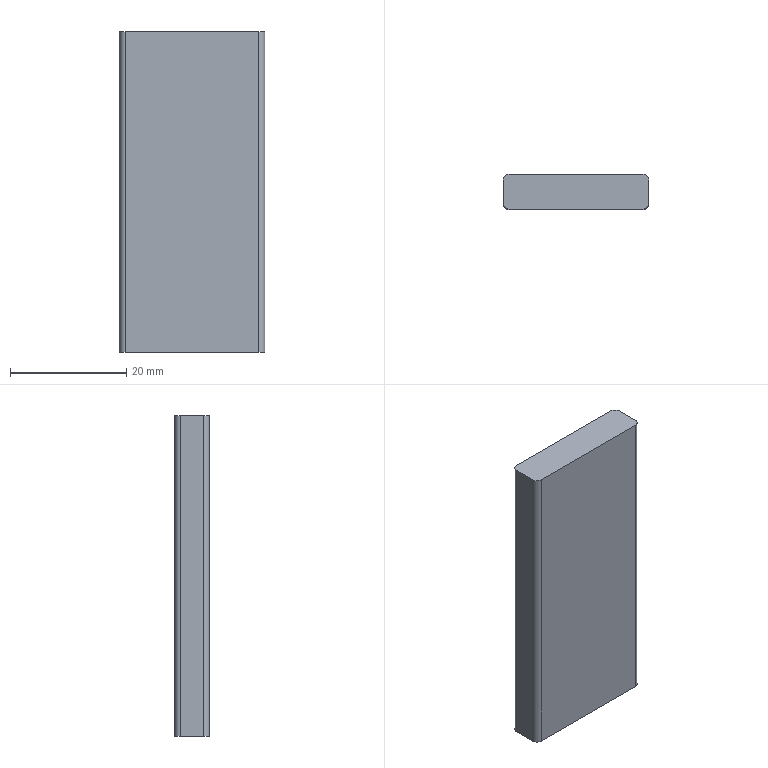Part | STEP file | 1 solid | 10 faces | box 24.97 x 5.97 x 55 mm | volume 8152 mm3 | plane 6 | cylinder 4 | commonest cylinder face diameters 2 x4
STEP:
#1=CARTESIAN_POINT('',(0.,0.,0.));
#2=DIRECTION('',(0.,0.,1.));
#3=DIRECTION('',(1.,0.,0.));
#4=AXIS2_PLACEMENT_3D('',#1,#2,#3);
#5=CARTESIAN_POINT('',(1790.232,496.365,31.619));
#6=VERTEX_POINT('',#5);
#7=CARTESIAN_POINT('',(1767.262,496.365,31.619));
#8=VERTEX_POINT('',#7);
#9=CARTESIAN_POINT('',(1791.247,496.365,31.619));
#10=DIRECTION('',(-1.,0.,0.));
#11=VECTOR('',#10,1.);
#12=LINE('',#9,#11);
#13=CARTESIAN_POINT('',(1801.247,562.98,31.619));
#14=DIRECTION('',(0.,0.,-1.));
#15=DIRECTION('',(-1.,0.,0.));
#16=AXIS2_PLACEMENT_3D('',#13,#14,#15);
#17=PLANE('',#16);
#18=CARTESIAN_POINT('',(10.,-66.615));
#19=DIRECTION('',(1.,0.));
#20=VECTOR('',#19,1.);
#21=LINE('',#18,#20);
#22=(GEOMETRIC_REPRESENTATION_CONTEXT(2)PARAMETRIC_REPRESENTATION_CONTEXT()REPRESENTATION_CONTEXT('',''));
#23=DEFINITIONAL_REPRESENTATION('',(#21),#22);
#24=PCURVE('',#17,#23);
#25=CARTESIAN_POINT('',(1791.247,496.365,426.119));
#26=DIRECTION('',(0.,-1.,0.));
#27=DIRECTION('',(0.,0.,1.));
#28=AXIS2_PLACEMENT_3D('',#25,#26,#27);
#29=PLANE('',#28);
#30=CARTESIAN_POINT('',(-394.5,0.));
#31=DIRECTION('',(0.,1.));
#32=VECTOR('',#31,1.);
#33=LINE('',#30,#32);
#34=(GEOMETRIC_REPRESENTATION_CONTEXT(2)PARAMETRIC_REPRESENTATION_CONTEXT()REPRESENTATION_CONTEXT('',''));
#35=DEFINITIONAL_REPRESENTATION('',(#33),#34);
#36=PCURVE('',#29,#35);
#37=SURFACE_CURVE('',#12,(#24,#36),.PCURVE_S1.);
#38=EDGE_CURVE('',#6,#8,#37,.T.);
#39=ORIENTED_EDGE('',*,*,#38,.T.);
#40=CARTESIAN_POINT('',(1766.262,495.365,31.619));
#41=VERTEX_POINT('',#40);
#42=CARTESIAN_POINT('',(1767.262,495.365,31.619));
#43=DIRECTION('',(0.,0.,1.));
#44=DIRECTION('',(-1.,0.,0.));
#45=AXIS2_PLACEMENT_3D('',#42,#43,#44);
#46=CIRCLE('',#45,1.);
#47=CARTESIAN_POINT('',(34.985,-67.615));
#48=CARTESIAN_POINT('',(34.985,-69.347));
#49=CARTESIAN_POINT('',(33.485,-68.481));
#50=CARTESIAN_POINT('',(31.985,-67.615));
#51=CARTESIAN_POINT('',(33.485,-66.749));
#52=CARTESIAN_POINT('',(34.985,-65.883));
#53=CARTESIAN_POINT('',(34.985,-67.615));
#54=(BOUNDED_CURVE()B_SPLINE_CURVE(2,(#47,#48,#49,#50,#51,#52,#53),.UNSPECIFIED.,.T.,.F.)B_SPLINE_CURVE_WITH_KNOTS((1,2,2,2,2,1),(-2.094,0.,2.094,4.189,6.283,8.378),.UNSPECIFIED.)CURVE()GEOMETRIC_REPRESENTATION_ITEM()RATIONAL_B_SPLINE_CURVE((1.,0.5,1.,0.5,1.,0.5,1.))REPRESENTATION_ITEM(''));
#55=(GEOMETRIC_REPRESENTATION_CONTEXT(2)PARAMETRIC_REPRESENTATION_CONTEXT()REPRESENTATION_CONTEXT('',''));
#56=DEFINITIONAL_REPRESENTATION('',(#54),#55);
#57=PCURVE('',#17,#56);
#58=CARTESIAN_POINT('',(1767.262,495.365,426.119));
#59=DIRECTION('',(0.,0.,-1.));
#60=DIRECTION('',(-1.,0.,0.));
#61=AXIS2_PLACEMENT_3D('',#58,#59,#60);
#62=CYLINDRICAL_SURFACE('',#61,1.);
#63=CARTESIAN_POINT('',(6.283,394.5));
#64=DIRECTION('',(-1.,0.));
#65=VECTOR('',#64,1.);
#66=LINE('',#63,#65);
#67=(GEOMETRIC_REPRESENTATION_CONTEXT(2)PARAMETRIC_REPRESENTATION_CONTEXT()REPRESENTATION_CONTEXT('',''));
#68=DEFINITIONAL_REPRESENTATION('',(#66),#67);
#69=PCURVE('',#62,#68);
#70=SURFACE_CURVE('',#46,(#57,#69),.PCURVE_S1.);
#71=EDGE_CURVE('',#8,#41,#70,.T.);
#72=ORIENTED_EDGE('',*,*,#71,.T.);
#73=CARTESIAN_POINT('',(1766.262,491.395,31.619));
#74=VERTEX_POINT('',#73);
#75=CARTESIAN_POINT('',(1766.262,496.38,31.619));
#76=DIRECTION('',(0.,-1.,0.));
#77=VECTOR('',#76,1.);
#78=LINE('',#75,#77);
#79=CARTESIAN_POINT('',(34.985,-66.6));
#80=DIRECTION('',(0.,-1.));
#81=VECTOR('',#80,1.);
#82=LINE('',#79,#81);
#83=(GEOMETRIC_REPRESENTATION_CONTEXT(2)PARAMETRIC_REPRESENTATION_CONTEXT()REPRESENTATION_CONTEXT('',''));
#84=DEFINITIONAL_REPRESENTATION('',(#82),#83);
#85=PCURVE('',#17,#84);
#86=CARTESIAN_POINT('',(1766.262,496.38,426.119));
#87=DIRECTION('',(1.,0.,0.));
#88=DIRECTION('',(0.,0.,-1.));
#89=AXIS2_PLACEMENT_3D('',#86,#87,#88);
#90=PLANE('',#89);
#91=CARTESIAN_POINT('',(394.5,0.));
#92=DIRECTION('',(0.,-1.));
#93=VECTOR('',#92,1.);
#94=LINE('',#91,#93);
#95=(GEOMETRIC_REPRESENTATION_CONTEXT(2)PARAMETRIC_REPRESENTATION_CONTEXT()REPRESENTATION_CONTEXT('',''));
#96=DEFINITIONAL_REPRESENTATION('',(#94),#95);
#97=PCURVE('',#90,#96);
#98=SURFACE_CURVE('',#78,(#85,#97),.PCURVE_S1.);
#99=EDGE_CURVE('',#41,#74,#98,.T.);
#100=ORIENTED_EDGE('',*,*,#99,.T.);
#101=CARTESIAN_POINT('',(1767.262,490.395,31.619));
#102=VERTEX_POINT('',#101);
#103=CARTESIAN_POINT('',(1767.262,491.395,31.619));
#104=DIRECTION('',(0.,0.,1.));
#105=DIRECTION('',(-1.,0.,0.));
#106=AXIS2_PLACEMENT_3D('',#103,#104,#105);
#107=CIRCLE('',#106,1.);
#108=CARTESIAN_POINT('',(34.985,-71.585));
#109=CARTESIAN_POINT('',(34.985,-73.317));
#110=CARTESIAN_POINT('',(33.485,-72.451));
#111=CARTESIAN_POINT('',(31.985,-71.585));
#112=CARTESIAN_POINT('',(33.485,-70.719));
#113=CARTESIAN_POINT('',(34.985,-69.853));
#114=CARTESIAN_POINT('',(34.985,-71.585));
#115=(BOUNDED_CURVE()B_SPLINE_CURVE(2,(#108,#109,#110,#111,#112,#113,#114),.UNSPECIFIED.,.T.,.F.)B_SPLINE_CURVE_WITH_KNOTS((1,2,2,2,2,1),(-2.094,0.,2.094,4.189,6.283,8.378),.UNSPECIFIED.)CURVE()GEOMETRIC_REPRESENTATION_ITEM()RATIONAL_B_SPLINE_CURVE((1.,0.5,1.,0.5,1.,0.5,1.))REPRESENTATION_ITEM(''));
#116=(GEOMETRIC_REPRESENTATION_CONTEXT(2)PARAMETRIC_REPRESENTATION_CONTEXT()REPRESENTATION_CONTEXT('',''));
#117=DEFINITIONAL_REPRESENTATION('',(#115),#116);
#118=PCURVE('',#17,#117);
#119=CARTESIAN_POINT('',(1767.262,491.395,426.119));
#120=DIRECTION('',(0.,0.,-1.));
#121=DIRECTION('',(-1.,0.,0.));
#122=AXIS2_PLACEMENT_3D('',#119,#120,#121);
#123=CYLINDRICAL_SURFACE('',#122,1.);
#124=CARTESIAN_POINT('',(6.283,394.5));
#125=DIRECTION('',(-1.,0.));
#126=VECTOR('',#125,1.);
#127=LINE('',#124,#126);
#128=(GEOMETRIC_REPRESENTATION_CONTEXT(2)PARAMETRIC_REPRESENTATION_CONTEXT()REPRESENTATION_CONTEXT('',''));
#129=DEFINITIONAL_REPRESENTATION('',(#127),#128);
#130=PCURVE('',#123,#129);
#131=SURFACE_CURVE('',#107,(#118,#130),.PCURVE_S1.);
#132=EDGE_CURVE('',#74,#102,#131,.T.);
#133=ORIENTED_EDGE('',*,*,#132,.T.);
#134=CARTESIAN_POINT('',(1790.232,490.395,31.619));
#135=VERTEX_POINT('',#134);
#136=CARTESIAN_POINT('',(1761.247,490.395,31.619));
#137=DIRECTION('',(1.,0.,0.));
#138=VECTOR('',#137,1.);
#139=LINE('',#136,#138);
#140=CARTESIAN_POINT('',(40.,-72.585));
#141=DIRECTION('',(-1.,0.));
#142=VECTOR('',#141,1.);
#143=LINE('',#140,#142);
#144=(GEOMETRIC_REPRESENTATION_CONTEXT(2)PARAMETRIC_REPRESENTATION_CONTEXT()REPRESENTATION_CONTEXT('',''));
#145=DEFINITIONAL_REPRESENTATION('',(#143),#144);
#146=PCURVE('',#17,#145);
#147=CARTESIAN_POINT('',(1761.247,490.395,426.119));
#148=DIRECTION('',(0.,1.,0.));
#149=DIRECTION('',(0.,0.,-1.));
#150=AXIS2_PLACEMENT_3D('',#147,#148,#149);
#151=PLANE('',#150);
#152=CARTESIAN_POINT('',(394.5,0.));
#153=DIRECTION('',(0.,-1.));
#154=VECTOR('',#153,1.);
#155=LINE('',#152,#154);
#156=(GEOMETRIC_REPRESENTATION_CONTEXT(2)PARAMETRIC_REPRESENTATION_CONTEXT()REPRESENTATION_CONTEXT('',''));
#157=DEFINITIONAL_REPRESENTATION('',(#155),#156);
#158=PCURVE('',#151,#157);
#159=SURFACE_CURVE('',#139,(#146,#158),.PCURVE_S1.);
#160=EDGE_CURVE('',#102,#135,#159,.T.);
#161=ORIENTED_EDGE('',*,*,#160,.T.);
#162=CARTESIAN_POINT('',(1791.232,491.395,31.619));
#163=VERTEX_POINT('',#162);
#164=CARTESIAN_POINT('',(1790.232,491.395,31.619));
#165=DIRECTION('',(0.,0.,1.));
#166=DIRECTION('',(-1.,0.,0.));
#167=AXIS2_PLACEMENT_3D('',#164,#165,#166);
#168=CIRCLE('',#167,1.);
#169=CARTESIAN_POINT('',(12.015,-71.585));
#170=CARTESIAN_POINT('',(12.015,-73.317));
#171=CARTESIAN_POINT('',(10.515,-72.451));
#172=CARTESIAN_POINT('',(9.015,-71.585));
#173=CARTESIAN_POINT('',(10.515,-70.719));
#174=CARTESIAN_POINT('',(12.015,-69.853));
#175=CARTESIAN_POINT('',(12.015,-71.585));
#176=(BOUNDED_CURVE()B_SPLINE_CURVE(2,(#169,#170,#171,#172,#173,#174,#175),.UNSPECIFIED.,.T.,.F.)B_SPLINE_CURVE_WITH_KNOTS((1,2,2,2,2,1),(-2.094,0.,2.094,4.189,6.283,8.378),.UNSPECIFIED.)CURVE()GEOMETRIC_REPRESENTATION_ITEM()RATIONAL_B_SPLINE_CURVE((1.,0.5,1.,0.5,1.,0.5,1.))REPRESENTATION_ITEM(''));
#177=(GEOMETRIC_REPRESENTATION_CONTEXT(2)PARAMETRIC_REPRESENTATION_CONTEXT()REPRESENTATION_CONTEXT('',''));
#178=DEFINITIONAL_REPRESENTATION('',(#176),#177);
#179=PCURVE('',#17,#178);
#180=CARTESIAN_POINT('',(1790.232,491.395,426.119));
#181=DIRECTION('',(0.,0.,-1.));
#182=DIRECTION('',(-1.,0.,0.));
#183=AXIS2_PLACEMENT_3D('',#180,#181,#182);
#184=CYLINDRICAL_SURFACE('',#183,1.);
#185=CARTESIAN_POINT('',(6.283,394.5));
#186=DIRECTION('',(-1.,0.));
#187=VECTOR('',#186,1.);
#188=LINE('',#185,#187);
#189=(GEOMETRIC_REPRESENTATION_CONTEXT(2)PARAMETRIC_REPRESENTATION_CONTEXT()REPRESENTATION_CONTEXT('',''));
#190=DEFINITIONAL_REPRESENTATION('',(#188),#189);
#191=PCURVE('',#184,#190);
#192=SURFACE_CURVE('',#168,(#179,#191),.PCURVE_S1.);
#193=EDGE_CURVE('',#135,#163,#192,.T.);
#194=ORIENTED_EDGE('',*,*,#193,.T.);
#195=CARTESIAN_POINT('',(1791.232,495.365,31.619));
#196=VERTEX_POINT('',#195);
#197=CARTESIAN_POINT('',(1791.232,490.38,31.619));
#198=DIRECTION('',(0.,1.,0.));
#199=VECTOR('',#198,1.);
#200=LINE('',#197,#199);
#201=CARTESIAN_POINT('',(10.015,-72.6));
#202=DIRECTION('',(0.,1.));
#203=VECTOR('',#202,1.);
#204=LINE('',#201,#203);
#205=(GEOMETRIC_REPRESENTATION_CONTEXT(2)PARAMETRIC_REPRESENTATION_CONTEXT()REPRESENTATION_CONTEXT('',''));
#206=DEFINITIONAL_REPRESENTATION('',(#204),#205);
#207=PCURVE('',#17,#206);
#208=CARTESIAN_POINT('',(1791.232,490.38,426.119));
#209=DIRECTION('',(-1.,0.,0.));
#210=DIRECTION('',(0.,0.,1.));
#211=AXIS2_PLACEMENT_3D('',#208,#209,#210);
#212=PLANE('',#211);
#213=CARTESIAN_POINT('',(-394.5,0.));
#214=DIRECTION('',(0.,1.));
#215=VECTOR('',#214,1.);
#216=LINE('',#213,#215);
#217=(GEOMETRIC_REPRESENTATION_CONTEXT(2)PARAMETRIC_REPRESENTATION_CONTEXT()REPRESENTATION_CONTEXT('',''));
#218=DEFINITIONAL_REPRESENTATION('',(#216),#217);
#219=PCURVE('',#212,#218);
#220=SURFACE_CURVE('',#200,(#207,#219),.PCURVE_S1.);
#221=EDGE_CURVE('',#163,#196,#220,.T.);
#222=ORIENTED_EDGE('',*,*,#221,.T.);
#223=CARTESIAN_POINT('',(1790.232,495.365,31.619));
#224=DIRECTION('',(0.,0.,1.));
#225=DIRECTION('',(-1.,0.,0.));
#226=AXIS2_PLACEMENT_3D('',#223,#224,#225);
#227=CIRCLE('',#226,1.);
#228=CARTESIAN_POINT('',(12.015,-67.615));
#229=CARTESIAN_POINT('',(12.015,-69.347));
#230=CARTESIAN_POINT('',(10.515,-68.481));
#231=CARTESIAN_POINT('',(9.015,-67.615));
#232=CARTESIAN_POINT('',(10.515,-66.749));
#233=CARTESIAN_POINT('',(12.015,-65.883));
#234=CARTESIAN_POINT('',(12.015,-67.615));
#235=(BOUNDED_CURVE()B_SPLINE_CURVE(2,(#228,#229,#230,#231,#232,#233,#234),.UNSPECIFIED.,.T.,.F.)B_SPLINE_CURVE_WITH_KNOTS((1,2,2,2,2,1),(-2.094,0.,2.094,4.189,6.283,8.378),.UNSPECIFIED.)CURVE()GEOMETRIC_REPRESENTATION_ITEM()RATIONAL_B_SPLINE_CURVE((1.,0.5,1.,0.5,1.,0.5,1.))REPRESENTATION_ITEM(''));
#236=(GEOMETRIC_REPRESENTATION_CONTEXT(2)PARAMETRIC_REPRESENTATION_CONTEXT()REPRESENTATION_CONTEXT('',''));
#237=DEFINITIONAL_REPRESENTATION('',(#235),#236);
#238=PCURVE('',#17,#237);
#239=CARTESIAN_POINT('',(1790.232,495.365,426.119));
#240=DIRECTION('',(0.,0.,-1.));
#241=DIRECTION('',(-1.,0.,0.));
#242=AXIS2_PLACEMENT_3D('',#239,#240,#241);
#243=CYLINDRICAL_SURFACE('',#242,1.);
#244=CARTESIAN_POINT('',(6.283,394.5));
#245=DIRECTION('',(-1.,0.));
#246=VECTOR('',#245,1.);
#247=LINE('',#244,#246);
#248=(GEOMETRIC_REPRESENTATION_CONTEXT(2)PARAMETRIC_REPRESENTATION_CONTEXT()REPRESENTATION_CONTEXT('',''));
#249=DEFINITIONAL_REPRESENTATION('',(#247),#248);
#250=PCURVE('',#243,#249);
#251=SURFACE_CURVE('',#227,(#238,#250),.PCURVE_S1.);
#252=EDGE_CURVE('',#196,#6,#251,.T.);
#253=ORIENTED_EDGE('',*,*,#252,.T.);
#254=EDGE_LOOP('',(#39,#72,#100,#133,#161,#194,#222,#253));
#255=FACE_BOUND('',#254,.T.);
#256=ADVANCED_FACE('',(#255),#17,.F.);
#257=CARTESIAN_POINT('',(1790.232,496.365,-23.381));
#258=VERTEX_POINT('',#257);
#259=CARTESIAN_POINT('',(1767.262,496.365,-23.381));
#260=VERTEX_POINT('',#259);
#261=CARTESIAN_POINT('',(1791.247,496.365,-23.381));
#262=DIRECTION('',(-1.,0.,0.));
#263=VECTOR('',#262,1.);
#264=LINE('',#261,#263);
#265=CARTESIAN_POINT('',(-449.5,0.));
#266=DIRECTION('',(0.,1.));
#267=VECTOR('',#266,1.);
#268=LINE('',#265,#267);
#269=(GEOMETRIC_REPRESENTATION_CONTEXT(2)PARAMETRIC_REPRESENTATION_CONTEXT()REPRESENTATION_CONTEXT('',''));
#270=DEFINITIONAL_REPRESENTATION('',(#268),#269);
#271=PCURVE('',#29,#270);
#272=CARTESIAN_POINT('',(18956.132,-3517.479,-23.381));
#273=DIRECTION('',(0.,0.,1.));
#274=DIRECTION('',(1.,0.,0.));
#275=AXIS2_PLACEMENT_3D('',#272,#273,#274);
#276=PLANE('',#275);
#277=CARTESIAN_POINT('',(-17164.884,4013.844));
#278=DIRECTION('',(-1.,0.));
#279=VECTOR('',#278,1.);
#280=LINE('',#277,#279);
#281=(GEOMETRIC_REPRESENTATION_CONTEXT(2)PARAMETRIC_REPRESENTATION_CONTEXT()REPRESENTATION_CONTEXT('',''));
#282=DEFINITIONAL_REPRESENTATION('',(#280),#281);
#283=PCURVE('',#276,#282);
#284=SURFACE_CURVE('',#264,(#271,#283),.PCURVE_S1.);
#285=EDGE_CURVE('',#258,#260,#284,.T.);
#286=ORIENTED_EDGE('',*,*,#285,.T.);
#287=CARTESIAN_POINT('',(1767.262,496.365,426.119));
#288=DIRECTION('',(0.,0.,1.));
#289=VECTOR('',#288,1.);
#290=LINE('',#287,#289);
#291=CARTESIAN_POINT('',(0.,23.985));
#292=DIRECTION('',(1.,0.));
#293=VECTOR('',#292,1.);
#294=LINE('',#291,#293);
#295=(GEOMETRIC_REPRESENTATION_CONTEXT(2)PARAMETRIC_REPRESENTATION_CONTEXT()REPRESENTATION_CONTEXT('',''));
#296=DEFINITIONAL_REPRESENTATION('',(#294),#295);
#297=PCURVE('',#29,#296);
#298=CARTESIAN_POINT('',(1.571,0.));
#299=DIRECTION('',(0.,-1.));
#300=VECTOR('',#299,1.);
#301=LINE('',#298,#300);
#302=(GEOMETRIC_REPRESENTATION_CONTEXT(2)PARAMETRIC_REPRESENTATION_CONTEXT()REPRESENTATION_CONTEXT('',''));
#303=DEFINITIONAL_REPRESENTATION('',(#301),#302);
#304=PCURVE('',#62,#303);
#305=SURFACE_CURVE('',#290,(#297,#304),.PCURVE_S1.);
#306=EDGE_CURVE('',#260,#8,#305,.T.);
#307=ORIENTED_EDGE('',*,*,#306,.T.);
#308=ORIENTED_EDGE('',*,*,#38,.F.);
#309=CARTESIAN_POINT('',(1790.232,496.365,426.119));
#310=DIRECTION('',(0.,0.,-1.));
#311=VECTOR('',#310,1.);
#312=LINE('',#309,#311);
#313=CARTESIAN_POINT('',(0.,1.015));
#314=DIRECTION('',(-1.,0.));
#315=VECTOR('',#314,1.);
#316=LINE('',#313,#315);
#317=(GEOMETRIC_REPRESENTATION_CONTEXT(2)PARAMETRIC_REPRESENTATION_CONTEXT()REPRESENTATION_CONTEXT('',''));
#318=DEFINITIONAL_REPRESENTATION('',(#316),#317);
#319=PCURVE('',#29,#318);
#320=CARTESIAN_POINT('',(1.571,0.));
#321=DIRECTION('',(0.,1.));
#322=VECTOR('',#321,1.);
#323=LINE('',#320,#322);
#324=(GEOMETRIC_REPRESENTATION_CONTEXT(2)PARAMETRIC_REPRESENTATION_CONTEXT()REPRESENTATION_CONTEXT('',''));
#325=DEFINITIONAL_REPRESENTATION('',(#323),#324);
#326=PCURVE('',#243,#325);
#327=SURFACE_CURVE('',#312,(#319,#326),.PCURVE_S1.);
#328=EDGE_CURVE('',#6,#258,#327,.T.);
#329=ORIENTED_EDGE('',*,*,#328,.T.);
#330=EDGE_LOOP('',(#286,#307,#308,#329));
#331=FACE_BOUND('',#330,.T.);
#332=ADVANCED_FACE('',(#331),#29,.F.);
#333=ORIENTED_EDGE('',*,*,#99,.F.);
#334=CARTESIAN_POINT('',(1766.262,495.365,-23.381));
#335=VERTEX_POINT('',#334);
#336=CARTESIAN_POINT('',(1766.262,495.365,426.119));
#337=DIRECTION('',(0.,0.,-1.));
#338=VECTOR('',#337,1.);
#339=LINE('',#336,#338);
#340=CARTESIAN_POINT('',(0.,-1.015));
#341=DIRECTION('',(1.,0.));
#342=VECTOR('',#341,1.);
#343=LINE('',#340,#342);
#344=(GEOMETRIC_REPRESENTATION_CONTEXT(2)PARAMETRIC_REPRESENTATION_CONTEXT()REPRESENTATION_CONTEXT('',''));
#345=DEFINITIONAL_REPRESENTATION('',(#343),#344);
#346=PCURVE('',#90,#345);
#347=CARTESIAN_POINT('',(0.,0.));
#348=DIRECTION('',(0.,1.));
#349=VECTOR('',#348,1.);
#350=LINE('',#347,#349);
#351=(GEOMETRIC_REPRESENTATION_CONTEXT(2)PARAMETRIC_REPRESENTATION_CONTEXT()REPRESENTATION_CONTEXT('',''));
#352=DEFINITIONAL_REPRESENTATION('',(#350),#351);
#353=PCURVE('',#62,#352);
#354=SURFACE_CURVE('',#339,(#346,#353),.PCURVE_S1.);
#355=EDGE_CURVE('',#41,#335,#354,.T.);
#356=ORIENTED_EDGE('',*,*,#355,.T.);
#357=CARTESIAN_POINT('',(1766.262,491.395,-23.381));
#358=VERTEX_POINT('',#357);
#359=CARTESIAN_POINT('',(1766.262,496.38,-23.381));
#360=DIRECTION('',(0.,-1.,0.));
#361=VECTOR('',#360,1.);
#362=LINE('',#359,#361);
#363=CARTESIAN_POINT('',(449.5,0.));
#364=DIRECTION('',(0.,-1.));
#365=VECTOR('',#364,1.);
#366=LINE('',#363,#365);
#367=(GEOMETRIC_REPRESENTATION_CONTEXT(2)PARAMETRIC_REPRESENTATION_CONTEXT()REPRESENTATION_CONTEXT('',''));
#368=DEFINITIONAL_REPRESENTATION('',(#366),#367);
#369=PCURVE('',#90,#368);
#370=CARTESIAN_POINT('',(-17189.869,4013.859));
#371=DIRECTION('',(0.,-1.));
#372=VECTOR('',#371,1.);
#373=LINE('',#370,#372);
#374=(GEOMETRIC_REPRESENTATION_CONTEXT(2)PARAMETRIC_REPRESENTATION_CONTEXT()REPRESENTATION_CONTEXT('',''));
#375=DEFINITIONAL_REPRESENTATION('',(#373),#374);
#376=PCURVE('',#276,#375);
#377=SURFACE_CURVE('',#362,(#369,#376),.PCURVE_S1.);
#378=EDGE_CURVE('',#335,#358,#377,.T.);
#379=ORIENTED_EDGE('',*,*,#378,.T.);
#380=CARTESIAN_POINT('',(1766.262,491.395,426.119));
#381=DIRECTION('',(0.,0.,1.));
#382=VECTOR('',#381,1.);
#383=LINE('',#380,#382);
#384=CARTESIAN_POINT('',(0.,-4.985));
#385=DIRECTION('',(-1.,0.));
#386=VECTOR('',#385,1.);
#387=LINE('',#384,#386);
#388=(GEOMETRIC_REPRESENTATION_CONTEXT(2)PARAMETRIC_REPRESENTATION_CONTEXT()REPRESENTATION_CONTEXT('',''));
#389=DEFINITIONAL_REPRESENTATION('',(#387),#388);
#390=PCURVE('',#90,#389);
#391=CARTESIAN_POINT('',(6.283,0.));
#392=DIRECTION('',(0.,-1.));
#393=VECTOR('',#392,1.);
#394=LINE('',#391,#393);
#395=(GEOMETRIC_REPRESENTATION_CONTEXT(2)PARAMETRIC_REPRESENTATION_CONTEXT()REPRESENTATION_CONTEXT('',''));
#396=DEFINITIONAL_REPRESENTATION('',(#394),#395);
#397=PCURVE('',#123,#396);
#398=SURFACE_CURVE('',#383,(#390,#397),.PCURVE_S1.);
#399=EDGE_CURVE('',#358,#74,#398,.T.);
#400=ORIENTED_EDGE('',*,*,#399,.T.);
#401=EDGE_LOOP('',(#333,#356,#379,#400));
#402=FACE_BOUND('',#401,.T.);
#403=ADVANCED_FACE('',(#402),#90,.F.);
#404=ORIENTED_EDGE('',*,*,#160,.F.);
#405=CARTESIAN_POINT('',(1767.262,490.395,-23.381));
#406=VERTEX_POINT('',#405);
#407=CARTESIAN_POINT('',(1767.262,490.395,426.119));
#408=DIRECTION('',(0.,0.,-1.));
#409=VECTOR('',#408,1.);
#410=LINE('',#407,#409);
#411=CARTESIAN_POINT('',(0.,-6.015));
#412=DIRECTION('',(1.,0.));
#413=VECTOR('',#412,1.);
#414=LINE('',#411,#413);
#415=(GEOMETRIC_REPRESENTATION_CONTEXT(2)PARAMETRIC_REPRESENTATION_CONTEXT()REPRESENTATION_CONTEXT('',''));
#416=DEFINITIONAL_REPRESENTATION('',(#414),#415);
#417=PCURVE('',#151,#416);
#418=CARTESIAN_POINT('',(4.712,0.));
#419=DIRECTION('',(0.,1.));
#420=VECTOR('',#419,1.);
#421=LINE('',#418,#420);
#422=(GEOMETRIC_REPRESENTATION_CONTEXT(2)PARAMETRIC_REPRESENTATION_CONTEXT()REPRESENTATION_CONTEXT('',''));
#423=DEFINITIONAL_REPRESENTATION('',(#421),#422);
#424=PCURVE('',#123,#423);
#425=SURFACE_CURVE('',#410,(#417,#424),.PCURVE_S1.);
#426=EDGE_CURVE('',#102,#406,#425,.T.);
#427=ORIENTED_EDGE('',*,*,#426,.T.);
#428=CARTESIAN_POINT('',(1790.232,490.395,-23.381));
#429=VERTEX_POINT('',#428);
#430=CARTESIAN_POINT('',(1761.247,490.395,-23.381));
#431=DIRECTION('',(1.,0.,0.));
#432=VECTOR('',#431,1.);
#433=LINE('',#430,#432);
#434=CARTESIAN_POINT('',(449.5,0.));
#435=DIRECTION('',(0.,-1.));
#436=VECTOR('',#435,1.);
#437=LINE('',#434,#436);
#438=(GEOMETRIC_REPRESENTATION_CONTEXT(2)PARAMETRIC_REPRESENTATION_CONTEXT()REPRESENTATION_CONTEXT('',''));
#439=DEFINITIONAL_REPRESENTATION('',(#437),#438);
#440=PCURVE('',#151,#439);
#441=CARTESIAN_POINT('',(-17194.884,4007.874));
#442=DIRECTION('',(1.,0.));
#443=VECTOR('',#442,1.);
#444=LINE('',#441,#443);
#445=(GEOMETRIC_REPRESENTATION_CONTEXT(2)PARAMETRIC_REPRESENTATION_CONTEXT()REPRESENTATION_CONTEXT('',''));
#446=DEFINITIONAL_REPRESENTATION('',(#444),#445);
#447=PCURVE('',#276,#446);
#448=SURFACE_CURVE('',#433,(#440,#447),.PCURVE_S1.);
#449=EDGE_CURVE('',#406,#429,#448,.T.);
#450=ORIENTED_EDGE('',*,*,#449,.T.);
#451=CARTESIAN_POINT('',(1790.232,490.395,426.119));
#452=DIRECTION('',(0.,0.,1.));
#453=VECTOR('',#452,1.);
#454=LINE('',#451,#453);
#455=CARTESIAN_POINT('',(0.,-28.985));
#456=DIRECTION('',(-1.,0.));
#457=VECTOR('',#456,1.);
#458=LINE('',#455,#457);
#459=(GEOMETRIC_REPRESENTATION_CONTEXT(2)PARAMETRIC_REPRESENTATION_CONTEXT()REPRESENTATION_CONTEXT('',''));
#460=DEFINITIONAL_REPRESENTATION('',(#458),#459);
#461=PCURVE('',#151,#460);
#462=CARTESIAN_POINT('',(4.712,0.));
#463=DIRECTION('',(0.,-1.));
#464=VECTOR('',#463,1.);
#465=LINE('',#462,#464);
#466=(GEOMETRIC_REPRESENTATION_CONTEXT(2)PARAMETRIC_REPRESENTATION_CONTEXT()REPRESENTATION_CONTEXT('',''));
#467=DEFINITIONAL_REPRESENTATION('',(#465),#466);
#468=PCURVE('',#184,#467);
#469=SURFACE_CURVE('',#454,(#461,#468),.PCURVE_S1.);
#470=EDGE_CURVE('',#429,#135,#469,.T.);
#471=ORIENTED_EDGE('',*,*,#470,.T.);
#472=EDGE_LOOP('',(#404,#427,#450,#471));
#473=FACE_BOUND('',#472,.T.);
#474=ADVANCED_FACE('',(#473),#151,.F.);
#475=CARTESIAN_POINT('',(1791.232,491.395,-23.381));
#476=VERTEX_POINT('',#475);
#477=CARTESIAN_POINT('',(1791.232,495.365,-23.381));
#478=VERTEX_POINT('',#477);
#479=CARTESIAN_POINT('',(1791.232,490.38,-23.381));
#480=DIRECTION('',(0.,1.,0.));
#481=VECTOR('',#480,1.);
#482=LINE('',#479,#481);
#483=CARTESIAN_POINT('',(-449.5,0.));
#484=DIRECTION('',(0.,1.));
#485=VECTOR('',#484,1.);
#486=LINE('',#483,#485);
#487=(GEOMETRIC_REPRESENTATION_CONTEXT(2)PARAMETRIC_REPRESENTATION_CONTEXT()REPRESENTATION_CONTEXT('',''));
#488=DEFINITIONAL_REPRESENTATION('',(#486),#487);
#489=PCURVE('',#212,#488);
#490=CARTESIAN_POINT('',(-17164.899,4007.859));
#491=DIRECTION('',(0.,1.));
#492=VECTOR('',#491,1.);
#493=LINE('',#490,#492);
#494=(GEOMETRIC_REPRESENTATION_CONTEXT(2)PARAMETRIC_REPRESENTATION_CONTEXT()REPRESENTATION_CONTEXT('',''));
#495=DEFINITIONAL_REPRESENTATION('',(#493),#494);
#496=PCURVE('',#276,#495);
#497=SURFACE_CURVE('',#482,(#489,#496),.PCURVE_S1.);
#498=EDGE_CURVE('',#476,#478,#497,.T.);
#499=ORIENTED_EDGE('',*,*,#498,.T.);
#500=CARTESIAN_POINT('',(1791.232,495.365,426.119));
#501=DIRECTION('',(0.,0.,1.));
#502=VECTOR('',#501,1.);
#503=LINE('',#500,#502);
#504=CARTESIAN_POINT('',(0.,4.985));
#505=DIRECTION('',(1.,0.));
#506=VECTOR('',#505,1.);
#507=LINE('',#504,#506);
#508=(GEOMETRIC_REPRESENTATION_CONTEXT(2)PARAMETRIC_REPRESENTATION_CONTEXT()REPRESENTATION_CONTEXT('',''));
#509=DEFINITIONAL_REPRESENTATION('',(#507),#508);
#510=PCURVE('',#212,#509);
#511=CARTESIAN_POINT('',(3.142,0.));
#512=DIRECTION('',(0.,-1.));
#513=VECTOR('',#512,1.);
#514=LINE('',#511,#513);
#515=(GEOMETRIC_REPRESENTATION_CONTEXT(2)PARAMETRIC_REPRESENTATION_CONTEXT()REPRESENTATION_CONTEXT('',''));
#516=DEFINITIONAL_REPRESENTATION('',(#514),#515);
#517=PCURVE('',#243,#516);
#518=SURFACE_CURVE('',#503,(#510,#517),.PCURVE_S1.);
#519=EDGE_CURVE('',#478,#196,#518,.T.);
#520=ORIENTED_EDGE('',*,*,#519,.T.);
#521=ORIENTED_EDGE('',*,*,#221,.F.);
#522=CARTESIAN_POINT('',(1791.232,491.395,426.119));
#523=DIRECTION('',(0.,0.,-1.));
#524=VECTOR('',#523,1.);
#525=LINE('',#522,#524);
#526=CARTESIAN_POINT('',(0.,1.015));
#527=DIRECTION('',(-1.,0.));
#528=VECTOR('',#527,1.);
#529=LINE('',#526,#528);
#530=(GEOMETRIC_REPRESENTATION_CONTEXT(2)PARAMETRIC_REPRESENTATION_CONTEXT()REPRESENTATION_CONTEXT('',''));
#531=DEFINITIONAL_REPRESENTATION('',(#529),#530);
#532=PCURVE('',#212,#531);
#533=CARTESIAN_POINT('',(3.142,0.));
#534=DIRECTION('',(0.,1.));
#535=VECTOR('',#534,1.);
#536=LINE('',#533,#535);
#537=(GEOMETRIC_REPRESENTATION_CONTEXT(2)PARAMETRIC_REPRESENTATION_CONTEXT()REPRESENTATION_CONTEXT('',''));
#538=DEFINITIONAL_REPRESENTATION('',(#536),#537);
#539=PCURVE('',#184,#538);
#540=SURFACE_CURVE('',#525,(#532,#539),.PCURVE_S1.);
#541=EDGE_CURVE('',#163,#476,#540,.T.);
#542=ORIENTED_EDGE('',*,*,#541,.T.);
#543=EDGE_LOOP('',(#499,#520,#521,#542));
#544=FACE_BOUND('',#543,.T.);
#545=ADVANCED_FACE('',(#544),#212,.F.);
#546=ORIENTED_EDGE('',*,*,#378,.F.);
#547=CARTESIAN_POINT('',(1767.262,495.365,-23.381));
#548=DIRECTION('',(0.,0.,-1.));
#549=DIRECTION('',(1.,0.,0.));
#550=AXIS2_PLACEMENT_3D('',#547,#548,#549);
#551=CIRCLE('',#550,1.);
#552=CARTESIAN_POINT('',(-17187.869,4012.844));
#553=CARTESIAN_POINT('',(-17187.869,4011.112));
#554=CARTESIAN_POINT('',(-17189.369,4011.978));
#555=CARTESIAN_POINT('',(-17190.869,4012.844));
#556=CARTESIAN_POINT('',(-17189.369,4013.71));
#557=CARTESIAN_POINT('',(-17187.869,4014.576));
#558=CARTESIAN_POINT('',(-17187.869,4012.844));
#559=(BOUNDED_CURVE()B_SPLINE_CURVE(2,(#552,#553,#554,#555,#556,#557,#558),.UNSPECIFIED.,.T.,.F.)B_SPLINE_CURVE_WITH_KNOTS((1,2,2,2,2,1),(-2.094,0.,2.094,4.189,6.283,8.378),.UNSPECIFIED.)CURVE()GEOMETRIC_REPRESENTATION_ITEM()RATIONAL_B_SPLINE_CURVE((1.,0.5,1.,0.5,1.,0.5,1.))REPRESENTATION_ITEM(''));
#560=(GEOMETRIC_REPRESENTATION_CONTEXT(2)PARAMETRIC_REPRESENTATION_CONTEXT()REPRESENTATION_CONTEXT('',''));
#561=DEFINITIONAL_REPRESENTATION('',(#559),#560);
#562=PCURVE('',#276,#561);
#563=CARTESIAN_POINT('',(-3.142,449.5));
#564=DIRECTION('',(1.,0.));
#565=VECTOR('',#564,1.);
#566=LINE('',#563,#565);
#567=(GEOMETRIC_REPRESENTATION_CONTEXT(2)PARAMETRIC_REPRESENTATION_CONTEXT()REPRESENTATION_CONTEXT('',''));
#568=DEFINITIONAL_REPRESENTATION('',(#566),#567);
#569=PCURVE('',#62,#568);
#570=SURFACE_CURVE('',#551,(#562,#569),.PCURVE_S1.);
#571=EDGE_CURVE('',#335,#260,#570,.T.);
#572=ORIENTED_EDGE('',*,*,#571,.T.);
#573=ORIENTED_EDGE('',*,*,#285,.F.);
#574=CARTESIAN_POINT('',(1790.232,495.365,-23.381));
#575=DIRECTION('',(0.,0.,-1.));
#576=DIRECTION('',(1.,0.,0.));
#577=AXIS2_PLACEMENT_3D('',#574,#575,#576);
#578=CIRCLE('',#577,1.);
#579=CARTESIAN_POINT('',(-17164.899,4012.844));
#580=CARTESIAN_POINT('',(-17164.899,4011.112));
#581=CARTESIAN_POINT('',(-17166.399,4011.978));
#582=CARTESIAN_POINT('',(-17167.899,4012.844));
#583=CARTESIAN_POINT('',(-17166.399,4013.71));
#584=CARTESIAN_POINT('',(-17164.899,4014.576));
#585=CARTESIAN_POINT('',(-17164.899,4012.844));
#586=(BOUNDED_CURVE()B_SPLINE_CURVE(2,(#579,#580,#581,#582,#583,#584,#585),.UNSPECIFIED.,.T.,.F.)B_SPLINE_CURVE_WITH_KNOTS((1,2,2,2,2,1),(-2.094,0.,2.094,4.189,6.283,8.378),.UNSPECIFIED.)CURVE()GEOMETRIC_REPRESENTATION_ITEM()RATIONAL_B_SPLINE_CURVE((1.,0.5,1.,0.5,1.,0.5,1.))REPRESENTATION_ITEM(''));
#587=(GEOMETRIC_REPRESENTATION_CONTEXT(2)PARAMETRIC_REPRESENTATION_CONTEXT()REPRESENTATION_CONTEXT('',''));
#588=DEFINITIONAL_REPRESENTATION('',(#586),#587);
#589=PCURVE('',#276,#588);
#590=CARTESIAN_POINT('',(-3.142,449.5));
#591=DIRECTION('',(1.,0.));
#592=VECTOR('',#591,1.);
#593=LINE('',#590,#592);
#594=(GEOMETRIC_REPRESENTATION_CONTEXT(2)PARAMETRIC_REPRESENTATION_CONTEXT()REPRESENTATION_CONTEXT('',''));
#595=DEFINITIONAL_REPRESENTATION('',(#593),#594);
#596=PCURVE('',#243,#595);
#597=SURFACE_CURVE('',#578,(#589,#596),.PCURVE_S1.);
#598=EDGE_CURVE('',#258,#478,#597,.T.);
#599=ORIENTED_EDGE('',*,*,#598,.T.);
#600=ORIENTED_EDGE('',*,*,#498,.F.);
#601=CARTESIAN_POINT('',(1790.232,491.395,-23.381));
#602=DIRECTION('',(0.,0.,-1.));
#603=DIRECTION('',(1.,0.,0.));
#604=AXIS2_PLACEMENT_3D('',#601,#602,#603);
#605=CIRCLE('',#604,1.);
#606=CARTESIAN_POINT('',(-17164.899,4008.874));
#607=CARTESIAN_POINT('',(-17164.899,4007.142));
#608=CARTESIAN_POINT('',(-17166.399,4008.008));
#609=CARTESIAN_POINT('',(-17167.899,4008.874));
#610=CARTESIAN_POINT('',(-17166.399,4009.74));
#611=CARTESIAN_POINT('',(-17164.899,4010.606));
#612=CARTESIAN_POINT('',(-17164.899,4008.874));
#613=(BOUNDED_CURVE()B_SPLINE_CURVE(2,(#606,#607,#608,#609,#610,#611,#612),.UNSPECIFIED.,.T.,.F.)B_SPLINE_CURVE_WITH_KNOTS((1,2,2,2,2,1),(-2.094,0.,2.094,4.189,6.283,8.378),.UNSPECIFIED.)CURVE()GEOMETRIC_REPRESENTATION_ITEM()RATIONAL_B_SPLINE_CURVE((1.,0.5,1.,0.5,1.,0.5,1.))REPRESENTATION_ITEM(''));
#614=(GEOMETRIC_REPRESENTATION_CONTEXT(2)PARAMETRIC_REPRESENTATION_CONTEXT()REPRESENTATION_CONTEXT('',''));
#615=DEFINITIONAL_REPRESENTATION('',(#613),#614);
#616=PCURVE('',#276,#615);
#617=CARTESIAN_POINT('',(3.142,449.5));
#618=DIRECTION('',(1.,0.));
#619=VECTOR('',#618,1.);
#620=LINE('',#617,#619);
#621=(GEOMETRIC_REPRESENTATION_CONTEXT(2)PARAMETRIC_REPRESENTATION_CONTEXT()REPRESENTATION_CONTEXT('',''));
#622=DEFINITIONAL_REPRESENTATION('',(#620),#621);
#623=PCURVE('',#184,#622);
#624=SURFACE_CURVE('',#605,(#616,#623),.PCURVE_S1.);
#625=EDGE_CURVE('',#476,#429,#624,.T.);
#626=ORIENTED_EDGE('',*,*,#625,.T.);
#627=ORIENTED_EDGE('',*,*,#449,.F.);
#628=CARTESIAN_POINT('',(1767.262,491.395,-23.381));
#629=DIRECTION('',(0.,0.,-1.));
#630=DIRECTION('',(1.,0.,0.));
#631=AXIS2_PLACEMENT_3D('',#628,#629,#630);
#632=CIRCLE('',#631,1.);
#633=CARTESIAN_POINT('',(-17187.869,4008.874));
#634=CARTESIAN_POINT('',(-17187.869,4007.142));
#635=CARTESIAN_POINT('',(-17189.369,4008.008));
#636=CARTESIAN_POINT('',(-17190.869,4008.874));
#637=CARTESIAN_POINT('',(-17189.369,4009.74));
#638=CARTESIAN_POINT('',(-17187.869,4010.606));
#639=CARTESIAN_POINT('',(-17187.869,4008.874));
#640=(BOUNDED_CURVE()B_SPLINE_CURVE(2,(#633,#634,#635,#636,#637,#638,#639),.UNSPECIFIED.,.T.,.F.)B_SPLINE_CURVE_WITH_KNOTS((1,2,2,2,2,1),(-2.094,0.,2.094,4.189,6.283,8.378),.UNSPECIFIED.)CURVE()GEOMETRIC_REPRESENTATION_ITEM()RATIONAL_B_SPLINE_CURVE((1.,0.5,1.,0.5,1.,0.5,1.))REPRESENTATION_ITEM(''));
#641=(GEOMETRIC_REPRESENTATION_CONTEXT(2)PARAMETRIC_REPRESENTATION_CONTEXT()REPRESENTATION_CONTEXT('',''));
#642=DEFINITIONAL_REPRESENTATION('',(#640),#641);
#643=PCURVE('',#276,#642);
#644=CARTESIAN_POINT('',(3.142,449.5));
#645=DIRECTION('',(1.,0.));
#646=VECTOR('',#645,1.);
#647=LINE('',#644,#646);
#648=(GEOMETRIC_REPRESENTATION_CONTEXT(2)PARAMETRIC_REPRESENTATION_CONTEXT()REPRESENTATION_CONTEXT('',''));
#649=DEFINITIONAL_REPRESENTATION('',(#647),#648);
#650=PCURVE('',#123,#649);
#651=SURFACE_CURVE('',#632,(#643,#650),.PCURVE_S1.);
#652=EDGE_CURVE('',#406,#358,#651,.T.);
#653=ORIENTED_EDGE('',*,*,#652,.T.);
#654=EDGE_LOOP('',(#546,#572,#573,#599,#600,#626,#627,#653));
#655=FACE_BOUND('',#654,.T.);
#656=ADVANCED_FACE('',(#655),#276,.F.);
#657=ORIENTED_EDGE('',*,*,#71,.F.);
#658=ORIENTED_EDGE('',*,*,#306,.F.);
#659=ORIENTED_EDGE('',*,*,#571,.F.);
#660=ORIENTED_EDGE('',*,*,#355,.F.);
#661=EDGE_LOOP('',(#657,#658,#659,#660));
#662=FACE_BOUND('',#661,.T.);
#663=ADVANCED_FACE('',(#662),#62,.T.);
#664=ORIENTED_EDGE('',*,*,#132,.F.);
#665=ORIENTED_EDGE('',*,*,#399,.F.);
#666=ORIENTED_EDGE('',*,*,#652,.F.);
#667=ORIENTED_EDGE('',*,*,#426,.F.);
#668=EDGE_LOOP('',(#664,#665,#666,#667));
#669=FACE_BOUND('',#668,.T.);
#670=ADVANCED_FACE('',(#669),#123,.T.);
#671=ORIENTED_EDGE('',*,*,#252,.F.);
#672=ORIENTED_EDGE('',*,*,#519,.F.);
#673=ORIENTED_EDGE('',*,*,#598,.F.);
#674=ORIENTED_EDGE('',*,*,#328,.F.);
#675=EDGE_LOOP('',(#671,#672,#673,#674));
#676=FACE_BOUND('',#675,.T.);
#677=ADVANCED_FACE('',(#676),#243,.T.);
#678=ORIENTED_EDGE('',*,*,#193,.F.);
#679=ORIENTED_EDGE('',*,*,#470,.F.);
#680=ORIENTED_EDGE('',*,*,#625,.F.);
#681=ORIENTED_EDGE('',*,*,#541,.F.);
#682=EDGE_LOOP('',(#678,#679,#680,#681));
#683=FACE_BOUND('',#682,.T.);
#684=ADVANCED_FACE('',(#683),#184,.T.);
#685=CLOSED_SHELL('',(#256,#332,#403,#474,#545,#656,#663,#670,#677,#684));
#686=MANIFOLD_SOLID_BREP('',#685);
#687=(LENGTH_UNIT()NAMED_UNIT(*)SI_UNIT(.MILLI.,.METRE.));
#688=UNCERTAINTY_MEASURE_WITH_UNIT(LENGTH_MEASURE(0.0000001),#687,'','');
#689=(NAMED_UNIT(*)PLANE_ANGLE_UNIT()SI_UNIT($,.RADIAN.));
#690=(NAMED_UNIT(*)SI_UNIT($,.STERADIAN.)SOLID_ANGLE_UNIT());
#691=(GEOMETRIC_REPRESENTATION_CONTEXT(3)GLOBAL_UNCERTAINTY_ASSIGNED_CONTEXT((#688))GLOBAL_UNIT_ASSIGNED_CONTEXT((#687,#689,#690))REPRESENTATION_CONTEXT('',''));
#692=ADVANCED_BREP_SHAPE_REPRESENTATION('',(#4,#686),#691);